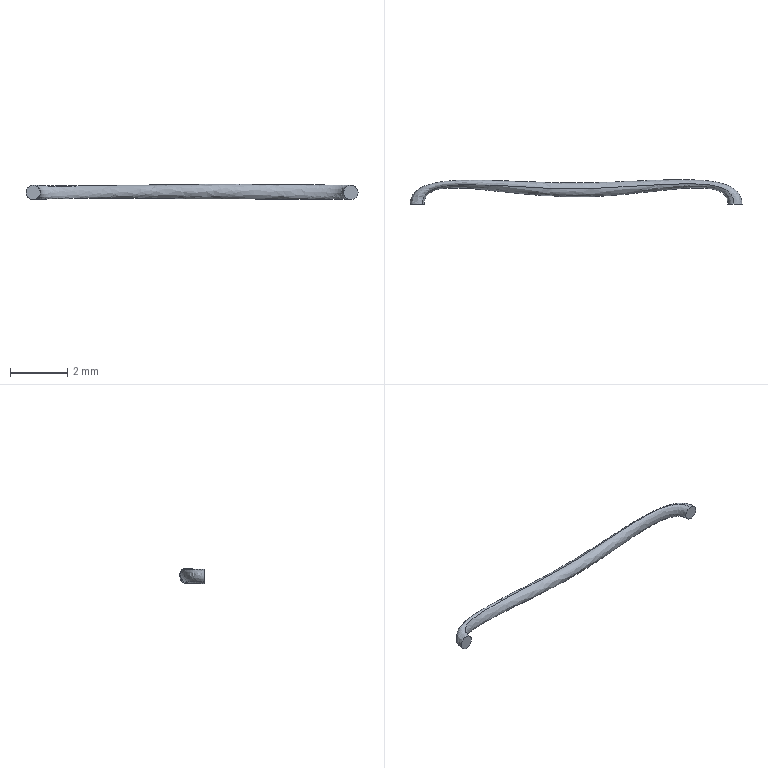Part | SolidWorks | features BaseBody 1 | 1 solid | 4 faces | box 11.637 x 0.8669 x 0.5347 mm | volume 1.747 mm3 | plane 2 | spline 2
STEP:
#1=CARTESIAN_POINT('',(347.519,424.469,93.88));
#2=VERTEX_POINT('',#1);
#3=CARTESIAN_POINT('',(347.463,424.469,94.377));
#4=VERTEX_POINT('',#3);
#5=CARTESIAN_POINT('',(347.519,424.469,93.88));
#6=CARTESIAN_POINT('',(347.553,424.469,93.884));
#7=CARTESIAN_POINT('',(347.618,424.47,93.905));
#8=CARTESIAN_POINT('',(347.691,424.47,93.969));
#9=CARTESIAN_POINT('',(347.737,424.47,94.055));
#10=CARTESIAN_POINT('',(347.746,424.47,94.15));
#11=CARTESIAN_POINT('',(347.722,424.47,94.236));
#12=CARTESIAN_POINT('',(347.663,424.47,94.322));
#13=CARTESIAN_POINT('',(347.588,424.469,94.366));
#14=CARTESIAN_POINT('',(347.524,424.469,94.377));
#15=CARTESIAN_POINT('',(347.504,424.469,94.379));
#16=CARTESIAN_POINT('',(347.484,424.469,94.379));
#17=CARTESIAN_POINT('',(347.47,424.469,94.378));
#18=CARTESIAN_POINT('',(347.463,424.469,94.377));
#19=B_SPLINE_CURVE_WITH_KNOTS('',3,(#5,#6,#7,#8,#9,#10,#11,#12,#13,#14,#15,#16,#17,#18),.UNSPECIFIED.,.F.,.F.,(4,1,1,1,1,1,1,1,1,1,1,4),(0.,0.125,0.25,0.375,0.5,0.6,0.7,0.9,0.925,0.95,0.975,1.),.UNSPECIFIED.);
#20=EDGE_CURVE('',#2,#4,#19,.T.);
#21=ORIENTED_EDGE('',*,*,#20,.T.);
#22=CARTESIAN_POINT('',(347.463,424.469,94.377));
#23=CARTESIAN_POINT('',(347.456,424.469,94.376));
#24=CARTESIAN_POINT('',(347.443,424.469,94.374));
#25=CARTESIAN_POINT('',(347.423,424.469,94.369));
#26=CARTESIAN_POINT('',(347.404,424.469,94.363));
#27=CARTESIAN_POINT('',(347.343,424.469,94.338));
#28=CARTESIAN_POINT('',(347.28,424.469,94.279));
#29=CARTESIAN_POINT('',(347.243,424.469,94.182));
#30=CARTESIAN_POINT('',(347.238,424.469,94.093));
#31=CARTESIAN_POINT('',(347.268,424.469,94.002));
#32=CARTESIAN_POINT('',(347.332,424.469,93.928));
#33=CARTESIAN_POINT('',(347.418,424.469,93.883));
#34=CARTESIAN_POINT('',(347.486,424.469,93.876));
#35=CARTESIAN_POINT('',(347.519,424.469,93.88));
#36=B_SPLINE_CURVE_WITH_KNOTS('',3,(#22,#23,#24,#25,#26,#27,#28,#29,#30,#31,#32,#33,#34,#35),.UNSPECIFIED.,.F.,.F.,(4,1,1,1,1,1,1,1,1,1,1,4),(0.,0.025,0.05,0.075,0.1,0.3,0.4,0.5,0.625,0.75,0.875,1.),.UNSPECIFIED.);
#37=EDGE_CURVE('',#4,#2,#36,.T.);
#38=ORIENTED_EDGE('',*,*,#37,.T.);
#39=EDGE_LOOP('',(#21,#38));
#40=FACE_OUTER_BOUND('',#39,.T.);
#41=CARTESIAN_POINT('',(347.491,424.469,94.129));
#42=DIRECTION('',(-0.0009599,1.,0.));
#43=DIRECTION('',(0.,0.,1.));
#44=AXIS2_PLACEMENT_3D('',#41,#42,#43);
#45=PLANE('',#44);
#46=ADVANCED_FACE('',(#40),#45,.F.);
#47=CARTESIAN_POINT('',(336.18,424.459,93.948));
#48=VERTEX_POINT('',#47);
#49=CARTESIAN_POINT('',(336.527,424.459,94.309));
#50=VERTEX_POINT('',#49);
#51=CARTESIAN_POINT('',(336.18,424.459,93.948));
#52=CARTESIAN_POINT('',(336.205,424.459,93.925));
#53=CARTESIAN_POINT('',(336.263,424.459,93.889));
#54=CARTESIAN_POINT('',(336.359,424.459,93.873));
#55=CARTESIAN_POINT('',(336.454,424.459,93.892));
#56=CARTESIAN_POINT('',(336.533,424.459,93.946));
#57=CARTESIAN_POINT('',(336.584,424.459,94.02));
#58=CARTESIAN_POINT('',(336.613,424.459,94.119));
#59=CARTESIAN_POINT('',(336.599,424.459,94.205));
#60=CARTESIAN_POINT('',(336.566,424.459,94.262));
#61=CARTESIAN_POINT('',(336.554,424.459,94.278));
#62=CARTESIAN_POINT('',(336.542,424.459,94.294));
#63=CARTESIAN_POINT('',(336.532,424.459,94.304));
#64=CARTESIAN_POINT('',(336.527,424.459,94.309));
#65=B_SPLINE_CURVE_WITH_KNOTS('',3,(#51,#52,#53,#54,#55,#56,#57,#58,#59,#60,#61,#62,#63,#64),.UNSPECIFIED.,.F.,.F.,(4,1,1,1,1,1,1,1,1,1,1,4),(0.,0.125,0.25,0.375,0.5,0.6,0.7,0.9,0.925,0.95,0.975,1.),.UNSPECIFIED.);
#66=EDGE_CURVE('',#48,#50,#65,.T.);
#67=ORIENTED_EDGE('',*,*,#66,.T.);
#68=CARTESIAN_POINT('',(336.527,424.459,94.309));
#69=CARTESIAN_POINT('',(336.522,424.459,94.313));
#70=CARTESIAN_POINT('',(336.512,424.459,94.322));
#71=CARTESIAN_POINT('',(336.496,424.459,94.335));
#72=CARTESIAN_POINT('',(336.479,424.459,94.345));
#73=CARTESIAN_POINT('',(336.421,424.459,94.376));
#74=CARTESIAN_POINT('',(336.335,424.459,94.387));
#75=CARTESIAN_POINT('',(336.236,424.459,94.354));
#76=CARTESIAN_POINT('',(336.165,424.459,94.301));
#77=CARTESIAN_POINT('',(336.114,424.458,94.22));
#78=CARTESIAN_POINT('',(336.098,424.458,94.124));
#79=CARTESIAN_POINT('',(336.118,424.458,94.028));
#80=CARTESIAN_POINT('',(336.156,424.459,93.972));
#81=CARTESIAN_POINT('',(336.18,424.459,93.948));
#82=B_SPLINE_CURVE_WITH_KNOTS('',3,(#68,#69,#70,#71,#72,#73,#74,#75,#76,#77,#78,#79,#80,#81),.UNSPECIFIED.,.F.,.F.,(4,1,1,1,1,1,1,1,1,1,1,4),(0.,0.025,0.05,0.075,0.1,0.3,0.4,0.5,0.625,0.75,0.875,1.),.UNSPECIFIED.);
#83=EDGE_CURVE('',#50,#48,#82,.T.);
#84=ORIENTED_EDGE('',*,*,#83,.T.);
#85=EDGE_LOOP('',(#67,#84));
#86=FACE_OUTER_BOUND('',#85,.T.);
#87=CARTESIAN_POINT('',(336.354,424.459,94.129));
#88=DIRECTION('',(-0.0009599,1.,0.));
#89=DIRECTION('',(0.,0.,1.));
#90=AXIS2_PLACEMENT_3D('',#87,#88,#89);
#91=PLANE('',#90);
#92=ADVANCED_FACE('',(#86),#91,.F.);
#93=CARTESIAN_POINT('',(336.18,424.459,93.948));
#94=CARTESIAN_POINT('',(336.179,425.673,93.948));
#95=CARTESIAN_POINT('',(341.995,424.193,93.907));
#96=CARTESIAN_POINT('',(347.518,425.655,93.88));
#97=CARTESIAN_POINT('',(347.519,424.469,93.88));
#98=B_SPLINE_CURVE_WITH_KNOTS('',3,(#93,#94,#95,#96,#97),.UNSPECIFIED.,.F.,.F.,(4,1,4),(0.,0.5,1.),.UNSPECIFIED.);
#99=EDGE_CURVE('',#48,#2,#98,.T.);
#100=ORIENTED_EDGE('',*,*,#99,.T.);
#101=ORIENTED_EDGE('',*,*,#37,.F.);
#102=CARTESIAN_POINT('',(347.463,424.469,94.377));
#103=CARTESIAN_POINT('',(347.462,425.654,94.377));
#104=CARTESIAN_POINT('',(341.849,424.365,94.469));
#105=CARTESIAN_POINT('',(336.526,425.615,94.309));
#106=CARTESIAN_POINT('',(336.527,424.459,94.309));
#107=B_SPLINE_CURVE_WITH_KNOTS('',3,(#102,#103,#104,#105,#106),.UNSPECIFIED.,.F.,.F.,(4,1,4),(0.,0.5,1.),.UNSPECIFIED.);
#108=EDGE_CURVE('',#4,#50,#107,.T.);
#109=ORIENTED_EDGE('',*,*,#108,.T.);
#110=ORIENTED_EDGE('',*,*,#66,.F.);
#111=EDGE_LOOP('',(#100,#101,#109,#110));
#112=FACE_OUTER_BOUND('',#111,.T.);
#113=CARTESIAN_POINT('',(336.179,424.338,93.959));
#114=CARTESIAN_POINT('',(335.986,425.723,93.961));
#115=CARTESIAN_POINT('',(342.005,424.171,93.896));
#116=CARTESIAN_POINT('',(347.721,425.709,93.882));
#117=CARTESIAN_POINT('',(347.525,424.342,93.882));
#118=CARTESIAN_POINT('',(336.182,424.338,93.956));
#119=CARTESIAN_POINT('',(335.99,425.722,93.957));
#120=CARTESIAN_POINT('',(342.005,424.162,93.9));
#121=CARTESIAN_POINT('',(347.716,425.708,93.881));
#122=CARTESIAN_POINT('',(347.52,424.342,93.881));
#123=CARTESIAN_POINT('',(336.209,424.339,93.928));
#124=CARTESIAN_POINT('',(336.017,425.713,93.928));
#125=CARTESIAN_POINT('',(342.011,424.095,93.927));
#126=CARTESIAN_POINT('',(347.676,425.697,93.874));
#127=CARTESIAN_POINT('',(347.482,424.343,93.876));
#128=CARTESIAN_POINT('',(336.271,424.341,93.889));
#129=CARTESIAN_POINT('',(336.082,425.695,93.885));
#130=CARTESIAN_POINT('',(342.017,423.975,93.996));
#131=CARTESIAN_POINT('',(347.6,425.677,93.879));
#132=CARTESIAN_POINT('',(347.408,424.345,93.883));
#133=CARTESIAN_POINT('',(336.367,424.344,93.873));
#134=CARTESIAN_POINT('',(336.181,425.668,93.865));
#135=CARTESIAN_POINT('',(342.012,423.858,94.117));
#136=CARTESIAN_POINT('',(347.511,425.652,93.922));
#137=CARTESIAN_POINT('',(347.323,424.348,93.929));
#138=CARTESIAN_POINT('',(336.462,424.347,93.893));
#139=CARTESIAN_POINT('',(336.28,425.644,93.881));
#140=CARTESIAN_POINT('',(341.995,423.793,94.247));
#141=CARTESIAN_POINT('',(347.446,425.634,93.994));
#142=CARTESIAN_POINT('',(347.259,424.35,94.002));
#143=CARTESIAN_POINT('',(336.541,424.348,93.947));
#144=CARTESIAN_POINT('',(336.362,425.626,93.933));
#145=CARTESIAN_POINT('',(341.969,423.794,94.368));
#146=CARTESIAN_POINT('',(347.416,425.625,94.084));
#147=CARTESIAN_POINT('',(347.229,424.351,94.093));
#148=CARTESIAN_POINT('',(336.592,424.349,94.02));
#149=CARTESIAN_POINT('',(336.415,425.619,94.006));
#150=CARTESIAN_POINT('',(341.939,423.851,94.457));
#151=CARTESIAN_POINT('',(347.421,425.628,94.173));
#152=CARTESIAN_POINT('',(347.233,424.35,94.182));
#153=CARTESIAN_POINT('',(336.621,424.349,94.12));
#154=CARTESIAN_POINT('',(336.446,425.618,94.107));
#155=CARTESIAN_POINT('',(341.904,423.967,94.525));
#156=CARTESIAN_POINT('',(347.461,425.641,94.271));
#157=CARTESIAN_POINT('',(347.271,424.349,94.279));
#158=CARTESIAN_POINT('',(336.606,424.348,94.205));
#159=CARTESIAN_POINT('',(336.432,425.628,94.195));
#160=CARTESIAN_POINT('',(341.878,424.104,94.534));
#161=CARTESIAN_POINT('',(347.528,425.662,94.331));
#162=CARTESIAN_POINT('',(347.334,424.347,94.338));
#163=CARTESIAN_POINT('',(336.574,424.346,94.262));
#164=CARTESIAN_POINT('',(336.399,425.641,94.254));
#165=CARTESIAN_POINT('',(341.863,424.218,94.508));
#166=CARTESIAN_POINT('',(347.591,425.68,94.358));
#167=CARTESIAN_POINT('',(347.395,424.345,94.363));
#168=CARTESIAN_POINT('',(336.562,424.346,94.279));
#169=CARTESIAN_POINT('',(336.387,425.645,94.271));
#170=CARTESIAN_POINT('',(341.859,424.253,94.499));
#171=CARTESIAN_POINT('',(347.611,425.686,94.365));
#172=CARTESIAN_POINT('',(347.414,424.344,94.37));
#173=CARTESIAN_POINT('',(336.55,424.345,94.294));
#174=CARTESIAN_POINT('',(336.374,425.65,94.288));
#175=CARTESIAN_POINT('',(341.855,424.288,94.487));
#176=CARTESIAN_POINT('',(347.631,425.692,94.37));
#177=CARTESIAN_POINT('',(347.433,424.343,94.374));
#178=CARTESIAN_POINT('',(336.537,424.345,94.308));
#179=CARTESIAN_POINT('',(336.361,425.654,94.303));
#180=CARTESIAN_POINT('',(341.852,424.32,94.474));
#181=CARTESIAN_POINT('',(347.651,425.698,94.374));
#182=CARTESIAN_POINT('',(347.452,424.343,94.377));
#183=CARTESIAN_POINT('',(336.528,424.345,94.316));
#184=CARTESIAN_POINT('',(336.352,425.657,94.311));
#185=CARTESIAN_POINT('',(341.85,424.341,94.465));
#186=CARTESIAN_POINT('',(347.663,425.702,94.375));
#187=CARTESIAN_POINT('',(347.464,424.342,94.378));
#188=CARTESIAN_POINT('',(336.524,424.344,94.319));
#189=CARTESIAN_POINT('',(336.348,425.659,94.315));
#190=CARTESIAN_POINT('',(341.849,424.35,94.461));
#191=CARTESIAN_POINT('',(347.668,425.703,94.375));
#192=CARTESIAN_POINT('',(347.469,424.342,94.378));
#193=B_SPLINE_SURFACE_WITH_KNOTS('',3,3,((#113,#114,#115,#116,#117),(#118,#119,#120,#121,#122),(#123,#124,#125,#126,#127),(#128,#129,#130,#131,#132),(#133,#134,#135,#136,#137),(#138,#139,#140,#141,#142),(#143,#144,#145,#146,#147),(#148,#149,#150,#151,#152),(#153,#154,#155,#156,#157),(#158,#159,#160,#161,#162),(#163,#164,#165,#166,#167),(#168,#169,#170,#171,#172),(#173,#174,#175,#176,#177),(#178,#179,#180,#181,#182),(#183,#184,#185,#186,#187),(#188,#189,#190,#191,#192)),.UNSPECIFIED.,.F.,.F.,.F.,(4,1,1,1,1,1,1,1,1,1,1,1,1,4),(4,1,4),(0.4905,0.5,0.5625,0.625,0.6875,0.75,0.8,0.85,0.95,0.9625,0.975,0.9875,1.,1.01),(-0.01567,0.5,1.017),.UNSPECIFIED.);
#194=ADVANCED_FACE('',(#112),#193,.F.);
#195=ORIENTED_EDGE('',*,*,#83,.F.);
#196=ORIENTED_EDGE('',*,*,#108,.F.);
#197=ORIENTED_EDGE('',*,*,#20,.F.);
#198=ORIENTED_EDGE('',*,*,#99,.F.);
#199=EDGE_LOOP('',(#195,#196,#197,#198));
#200=FACE_OUTER_BOUND('',#199,.T.);
#201=CARTESIAN_POINT('',(336.546,424.345,94.298));
#202=CARTESIAN_POINT('',(336.371,425.651,94.292));
#203=CARTESIAN_POINT('',(341.854,424.296,94.484));
#204=CARTESIAN_POINT('',(347.636,425.694,94.371));
#205=CARTESIAN_POINT('',(347.438,424.343,94.375));
#206=CARTESIAN_POINT('',(336.543,424.345,94.302));
#207=CARTESIAN_POINT('',(336.367,425.652,94.296));
#208=CARTESIAN_POINT('',(341.853,424.305,94.48));
#209=CARTESIAN_POINT('',(347.641,425.695,94.372));
#210=CARTESIAN_POINT('',(347.443,424.343,94.376));
#211=CARTESIAN_POINT('',(336.534,424.345,94.31));
#212=CARTESIAN_POINT('',(336.358,425.655,94.305));
#213=CARTESIAN_POINT('',(341.851,424.326,94.472));
#214=CARTESIAN_POINT('',(347.654,425.699,94.374));
#215=CARTESIAN_POINT('',(347.455,424.342,94.377));
#216=CARTESIAN_POINT('',(336.52,424.344,94.323));
#217=CARTESIAN_POINT('',(336.344,425.66,94.318));
#218=CARTESIAN_POINT('',(341.849,424.358,94.457));
#219=CARTESIAN_POINT('',(347.674,425.705,94.376));
#220=CARTESIAN_POINT('',(347.474,424.342,94.379));
#221=CARTESIAN_POINT('',(336.504,424.344,94.335));
#222=CARTESIAN_POINT('',(336.327,425.665,94.331));
#223=CARTESIAN_POINT('',(341.847,424.391,94.44));
#224=CARTESIAN_POINT('',(347.694,425.711,94.376));
#225=CARTESIAN_POINT('',(347.494,424.341,94.379));
#226=CARTESIAN_POINT('',(336.487,424.343,94.345));
#227=CARTESIAN_POINT('',(336.31,425.671,94.343));
#228=CARTESIAN_POINT('',(341.845,424.423,94.421));
#229=CARTESIAN_POINT('',(347.715,425.717,94.375));
#230=CARTESIAN_POINT('',(347.514,424.341,94.377));
#231=CARTESIAN_POINT('',(336.429,424.341,94.376));
#232=CARTESIAN_POINT('',(336.25,425.689,94.377));
#233=CARTESIAN_POINT('',(341.841,424.524,94.355));
#234=CARTESIAN_POINT('',(347.782,425.737,94.366));
#235=CARTESIAN_POINT('',(347.579,424.338,94.366));
#236=CARTESIAN_POINT('',(336.343,424.339,94.387));
#237=CARTESIAN_POINT('',(336.161,425.714,94.391));
#238=CARTESIAN_POINT('',(341.847,424.623,94.246));
#239=CARTESIAN_POINT('',(347.859,425.759,94.325));
#240=CARTESIAN_POINT('',(347.653,424.336,94.322));
#241=CARTESIAN_POINT('',(336.245,424.336,94.354));
#242=CARTESIAN_POINT('',(336.059,425.739,94.362));
#243=CARTESIAN_POINT('',(341.869,424.671,94.107));
#244=CARTESIAN_POINT('',(347.919,425.775,94.24));
#245=CARTESIAN_POINT('',(347.712,424.334,94.236));
#246=CARTESIAN_POINT('',(336.174,424.335,94.3));
#247=CARTESIAN_POINT('',(335.984,425.753,94.31));
#248=CARTESIAN_POINT('',(341.894,424.665,93.997));
#249=CARTESIAN_POINT('',(347.943,425.78,94.155));
#250=CARTESIAN_POINT('',(347.736,424.334,94.15));
#251=CARTESIAN_POINT('',(336.123,424.334,94.219));
#252=CARTESIAN_POINT('',(335.931,425.758,94.229));
#253=CARTESIAN_POINT('',(341.926,424.6,93.905));
#254=CARTESIAN_POINT('',(347.933,425.774,94.06));
#255=CARTESIAN_POINT('',(347.727,424.335,94.055));
#256=CARTESIAN_POINT('',(336.107,424.335,94.123));
#257=CARTESIAN_POINT('',(335.913,425.754,94.132));
#258=CARTESIAN_POINT('',(341.959,424.479,93.854));
#259=CARTESIAN_POINT('',(347.885,425.757,93.973));
#260=CARTESIAN_POINT('',(347.681,424.336,93.969));
#261=CARTESIAN_POINT('',(336.126,424.336,94.028));
#262=CARTESIAN_POINT('',(335.933,425.74,94.034));
#263=CARTESIAN_POINT('',(341.988,424.323,93.85));
#264=CARTESIAN_POINT('',(347.808,425.732,93.907));
#265=CARTESIAN_POINT('',(347.608,424.339,93.905));
#266=CARTESIAN_POINT('',(336.168,424.338,93.967));
#267=CARTESIAN_POINT('',(335.975,425.726,93.97));
#268=CARTESIAN_POINT('',(342.003,424.193,93.885));
#269=CARTESIAN_POINT('',(347.735,425.713,93.882));
#270=CARTESIAN_POINT('',(347.538,424.341,93.882));
#271=CARTESIAN_POINT('',(336.197,424.339,93.941));
#272=CARTESIAN_POINT('',(336.005,425.717,93.942));
#273=CARTESIAN_POINT('',(342.008,424.126,93.915));
#274=CARTESIAN_POINT('',(347.695,425.702,93.878));
#275=CARTESIAN_POINT('',(347.5,424.343,93.879));
#276=CARTESIAN_POINT('',(336.201,424.339,93.938));
#277=CARTESIAN_POINT('',(336.009,425.716,93.939));
#278=CARTESIAN_POINT('',(342.009,424.118,93.919));
#279=CARTESIAN_POINT('',(347.689,425.701,93.878));
#280=CARTESIAN_POINT('',(347.494,424.343,93.879));
#281=B_SPLINE_SURFACE_WITH_KNOTS('',3,3,((#201,#202,#203,#204,#205),(#206,#207,#208,#209,#210),(#211,#212,#213,#214,#215),(#216,#217,#218,#219,#220),(#221,#222,#223,#224,#225),(#226,#227,#228,#229,#230),(#231,#232,#233,#234,#235),(#236,#237,#238,#239,#240),(#241,#242,#243,#244,#245),(#246,#247,#248,#249,#250),(#251,#252,#253,#254,#255),(#256,#257,#258,#259,#260),(#261,#262,#263,#264,#265),(#266,#267,#268,#269,#270),(#271,#272,#273,#274,#275),(#276,#277,#278,#279,#280)),.UNSPECIFIED.,.F.,.F.,.F.,(4,1,1,1,1,1,1,1,1,1,1,1,1,4),(4,1,4),(-0.009538,0.,0.0125,0.025,0.0375,0.05,0.15,0.2,0.25,0.3125,0.375,0.4375,0.5,0.5095),(-0.01567,0.5,1.017),.UNSPECIFIED.);
#282=ADVANCED_FACE('',(#200),#281,.F.);
#283=CLOSED_SHELL('',(#46,#92,#194,#282));
#284=MANIFOLD_SOLID_BREP('',#283);
#285=CARTESIAN_POINT('',(0.,0.,0.));
#286=DIRECTION('',(0.,0.,1.));
#287=DIRECTION('',(1.,0.,0.));
#288=AXIS2_PLACEMENT_3D('',#285,#286,#287);
#289=(LENGTH_UNIT()NAMED_UNIT(*)SI_UNIT(.MILLI.,.METRE.));
#290=UNCERTAINTY_MEASURE_WITH_UNIT(LENGTH_MEASURE(0.00001),#289,'','');
#291=(NAMED_UNIT(*)PLANE_ANGLE_UNIT()SI_UNIT($,.RADIAN.));
#292=(NAMED_UNIT(*)SI_UNIT($,.STERADIAN.)SOLID_ANGLE_UNIT());
#293=(GEOMETRIC_REPRESENTATION_CONTEXT(3)GLOBAL_UNCERTAINTY_ASSIGNED_CONTEXT((#290))GLOBAL_UNIT_ASSIGNED_CONTEXT((#289,#291,#292))REPRESENTATION_CONTEXT('',''));
#294=ADVANCED_BREP_SHAPE_REPRESENTATION('',(#284,#288),#293);